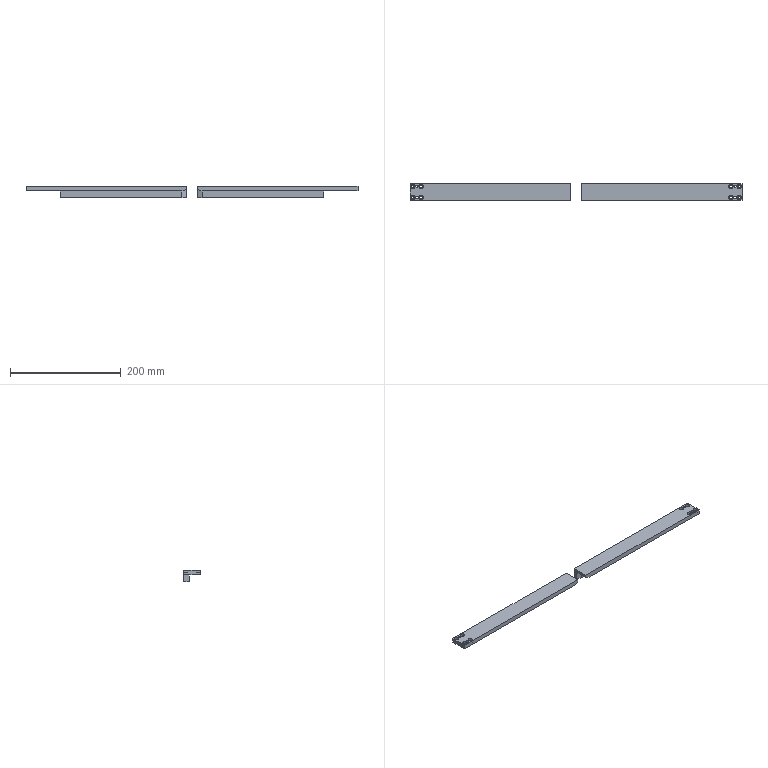NC program | NX | posted with a generic post | part box 600 x 30 x 20 mm
Lines 1 to 376 of 2978:
N10 G17 G21 G94 G90
(FLOOR_WALL , TOOL : D50)
N12 T01 M6
N14 G54
N16 G17 G0 G90 X-176. Y0. S6500 M3
N18 G43 Z30. H1
N20 Z3.
N22 G94 G1 Z0. F1250.
N24 X-173.
N26 X173.
N28 X176.
N30 Z3.
N32 G0 Z30.
N34 M5
(DRILLING_COPY_1 , TOOL : D6A45)
N36 T02 M6
N38 G54
N40 G17 G0 G90 X-140. Y-10. S3000 M3
N42 G43 Z30. H2
N44 G94 G81 G98 Z-1.6 F200. R3.
N46 X-132.5 Y-9.5
N48 X-125. Y-10.
N50 Y10.
N52 X-132.5
N54 X-140.
N56 G80
N58 G0 X-140. Y10. Z30.
N60 M5
(DRILLING_COPY_1_COPY_COPY_1_COPY_1_COPY , TOOL : 4.5ZT)
N62 T14 M6
N64 G54
N66 G17 G0 G90 X-140. Y10. S2000 M3
N68 G43 Z30. H14
N70 G94 G83 G98 Z-10.852 F120. Q2. R3.
N72 X-125.
N74 X-140. Y-10.
N76 X-125.
N78 G80
N80 G0 X-125. Y-10. Z30.
N82 M5
(DRILLING_COPY_1_COPY_COPY_1_COPY_1_COPY_COPY , TOOL : 2.5ZT)
N84 T12 M6
N86 G54
N88 G17 G0 G90 X-132.5 Y10. S2000 M3
N90 G43 Z30. H12
N92 G94 G83 G98 Z-10.251 F120. Q2. R3.
N94 Y-9.5
N96 G80
N98 G0 X-132.5 Y-9.5 Z30.
N100 M5
(ZLEVEL_PROFILE , TOOL : D10)
N102 T03 M6
N104 G54
N106 G17 G0 G90 X-47.703 Y20.1 S7000 M3
N108 G43 Z30. H3
N110 Z1.5
N112 G94 G1 X0. Z-1. F1000.
N114 X145. F3000.
N116 G2 X150.1 Y15. R5.1
N118 G1 Y-15.
N120 G2 X145. Y-20.1 R5.1
N122 G1 X-145.
N124 G2 X-150.1 Y-15. R5.1
N126 G1 Y15.
N128 G2 X-145. Y20.1 R5.1
N130 G1 X0.
N132 X57.29 Z-2.
N134 X145.
N136 G2 X150.1 Y15. R5.1
N138 G1 Y-15.
N140 G2 X145. Y-20.1 R5.1
N142 G1 X-145.
N144 G2 X-150.1 Y-15. R5.1
N146 G1 Y15.
N148 G2 X-145. Y20.1 R5.1
N150 G1 X0.
N152 X57.29 Z-3.
N154 X145.
N156 G2 X150.1 Y15. R5.1
N158 G1 Y-15.
N160 G2 X145. Y-20.1 R5.1
N162 G1 X-145.
N164 G2 X-150.1 Y-15. R5.1
N166 G1 Y15.
N168 G2 X-145. Y20.1 R5.1
N170 G1 X0.
N172 X57.29 Z-4.
N174 X145.
N176 G2 X150.1 Y15. R5.1
N178 G1 Y-15.
N180 G2 X145. Y-20.1 R5.1
N182 G1 X-145.
N184 G2 X-150.1 Y-15. R5.1
N186 G1 Y15.
N188 G2 X-145. Y20.1 R5.1
N190 G1 X0.
N192 X57.29 Z-5.
N194 X145.
N196 G2 X150.1 Y15. R5.1
N198 G1 Y-15.
N200 G2 X145. Y-20.1 R5.1
N202 G1 X-145.
N204 G2 X-150.1 Y-15. R5.1
N206 G1 Y15.
N208 G2 X-145. Y20.1 R5.1
N210 G1 X0.
N212 X57.29 Z-6.
N214 X145.
N216 G2 X150.1 Y15. R5.1
N218 G1 Y-15.
N220 G2 X145. Y-20.1 R5.1
N222 G1 X-145.
N224 G2 X-150.1 Y-15. R5.1
N226 G1 Y15.
N228 G2 X-145. Y20.1 R5.1
N230 G1 X0.
N232 X57.29 Z-7.
N234 X145.
N236 G2 X150.1 Y15. R5.1
N238 G1 Y-15.
N240 G2 X145. Y-20.1 R5.1
N242 G1 X-145.
N244 G2 X-150.1 Y-15. R5.1
N246 G1 Y15.
N248 G2 X-145. Y20.1 R5.1
N250 G1 X0.
N252 X57.29 Z-8.
N254 X145.
N256 G2 X150.1 Y15. R5.1
N258 G1 Y-15.
N260 G2 X145. Y-20.1 R5.1
N262 G1 X-145.
N264 G2 X-150.1 Y-15. R5.1
N266 G1 Y15.
N268 G2 X-145. Y20.1 R5.1
N270 G1 X0.
N272 X57.29 Z-9.
N274 X145.
N276 G2 X150.1 Y15. R5.1
N278 G1 Y-15.
N280 G2 X145. Y-20.1 R5.1
N282 G1 X-145.
N284 G2 X-150.1 Y-15. R5.1
N286 G1 Y15.
N288 G2 X-145. Y20.1 R5.1
N290 G1 X0.
N292 X57.29 Z-10.
N294 X145.
N296 G2 X150.1 Y15. R5.1
N298 G1 Y-15.
N300 G2 X145. Y-20.1 R5.1
N302 G1 X-145.
N304 G2 X-150.1 Y-15. R5.1
N306 G1 Y15.
N308 G2 X-145. Y20.1 R5.1
N310 G1 X0.
N312 X57.29 Z-11.
N314 X145.
N316 G2 X150.1 Y15. R5.1
N318 G1 Y-15.
N320 G2 X145. Y-20.1 R5.1
N322 G1 X-145.
N324 G2 X-150.1 Y-15. R5.1
N326 G1 Y15.
N328 G2 X-145. Y20.1 R5.1
N330 G1 X0.
N332 X57.29 Z-12.
N334 X145.
N336 G2 X150.1 Y15. R5.1
N338 G1 Y-15.
N340 G2 X145. Y-20.1 R5.1
N342 G1 X-145.
N344 G2 X-150.1 Y-15. R5.1
N346 G1 Y15.
N348 G2 X-145. Y20.1 R5.1
N350 G1 X0.
N352 X57.29 Z-13.
N354 X145.
N356 G2 X150.1 Y15. R5.1
N358 G1 Y-15.
N360 G2 X145. Y-20.1 R5.1
N362 G1 X-145.
N364 G2 X-150.1 Y-15. R5.1
N366 G1 Y15.
N368 G2 X-145. Y20.1 R5.1
N370 G1 X0.
N372 X57.29 Z-14.
N374 X145.
N376 G2 X150.1 Y15. R5.1
N378 G1 Y-15.
N380 G2 X145. Y-20.1 R5.1
N382 G1 X-145.
N384 G2 X-150.1 Y-15. R5.1
N386 G1 Y15.
N388 G2 X-145. Y20.1 R5.1
N390 G1 X0.
N392 X57.29 Z-15.
N394 X145.
N396 G2 X150.1 Y15. R5.1
N398 G1 Y-15.
N400 G2 X145. Y-20.1 R5.1
N402 G1 X-145.
N404 G2 X-150.1 Y-15. R5.1
N406 G1 Y15.
N408 G2 X-145. Y20.1 R5.1
N410 G1 X0.
N412 X57.29 Z-16.
N414 X145.
N416 G2 X150.1 Y15. R5.1
N418 G1 Y-15.
N420 G2 X145. Y-20.1 R5.1
N422 G1 X-145.
N424 G2 X-150.1 Y-15. R5.1
N426 G1 Y15.
N428 G2 X-145. Y20.1 R5.1
N430 G1 X0.
N432 X57.29 Z-17.
N434 X145.
N436 G2 X150.1 Y15. R5.1
N438 G1 Y-15.
N440 G2 X145. Y-20.1 R5.1
N442 G1 X-145.
N444 G2 X-150.1 Y-15. R5.1
N446 G1 Y15.
N448 G2 X-145. Y20.1 R5.1
N450 G1 X0.
N452 X57.29 Z-18.
N454 X145.
N456 G2 X150.1 Y15. R5.1
N458 G1 Y-15.
N460 G2 X145. Y-20.1 R5.1
N462 G1 X-145.
N464 G2 X-150.1 Y-15. R5.1
N466 G1 Y15.
N468 G2 X-145. Y20.1 R5.1
N470 G1 X0.
N472 X57.29 Z-19.
N474 X145.
N476 G2 X150.1 Y15. R5.1
N478 G1 Y-15.
N480 G2 X145. Y-20.1 R5.1
N482 G1 X-145.
N484 G2 X-150.1 Y-15. R5.1
N486 G1 Y15.
N488 G2 X-145. Y20.1 R5.1
N490 G1 X0.
N492 X57.29 Z-20.
N494 X145.
N496 G2 X150.1 Y15. R5.1
N498 G1 Y-15.
N500 G2 X145. Y-20.1 R5.1
N502 G1 X-145.
N504 G2 X-150.1 Y-15. R5.1
N506 G1 Y15.
N508 G2 X-145. Y20.1 R5.1
N510 G1 X57.29
N512 Z-18.5
N514 G0 Z30.
N516 M5
(ZLEVEL_PROFILE_COPY_COPY_1_COPY_COPY_COPY_1 , TOOL : D10JING)
N518 T04 M6
N520 G54
N522 G17 G0 G90 X146.096 Y-20.899 S7000 M3
N524 G43 Z30. H4
N526 Z-20.
N528 G94 G1 X145.866 Y-20.5 F1000.
N530 G3 X145. Y-20. R1.
N532 G1 X-145.
N534 G2 X-150. Y-15. R5.
N536 G1 Y15.
N538 G2 X-145. Y20. R5.
N540 G1 X145.
N542 G2 X150. Y15. R5.
N544 G1 Y-15.
N546 G2 X145. Y-20. R5.
N548 G3 X144.134 Y-20.5 R1.
N550 G1 X143.845 Y-21.
N552 G0 Z30.
N554 M5
(HOLE_MILLING_1 , TOOL : D6)
N556 T08 M6
N558 G54
N560 G17 G0 G90 X-140. Y10. S7000 M3
N562 G43 Z30. H8
N564 Z0.5
N566 G94 G3 X-139.5 Y9.5 R0.5 F1500.
N568 X-139. Y10. R0.5
N570 X-139. Y10. Z0. I-1. J0.
N572 X-139. Y10. Z-0.5 I-1. J0.
N574 X-139. Y10. Z-1. I-1. J0.
N576 X-139. Y10. Z-1.5 I-1. J0.
N578 X-139. Y10. Z-2. I-1. J0.
N580 X-139. Y10. Z-2.5 I-1. J0.
N582 X-139. Y10. Z-3. I-1. J0.
N584 X-139. Y10. Z-3.5 I-1. J0.
N586 X-139. Y10. Z-4. I-1. J0.
N588 X-139.691 Y9.049 Z-4.4 R-1.
N590 X-139.049 Y10.309 R1.
N592 X-139.691 Y9.049 R-1.
N594 X-139.37 Y9.679 R0.5
N596 X-140. Y10. R0.5
N598 G0 Z30.
N600 X-125.
N602 Z0.5
N604 G3 X-124.5 Y9.5 R0.5
N606 X-124. Y10. R0.5
N608 X-124. Y10. Z0. I-1. J0.
N610 X-124. Y10. Z-0.5 I-1. J0.
N612 X-124. Y10. Z-1. I-1. J0.
N614 X-124. Y10. Z-1.5 I-1. J0.
N616 X-124. Y10. Z-2. I-1. J0.
N618 X-124. Y10. Z-2.5 I-1. J0.
N620 X-124. Y10. Z-3. I-1. J0.
N622 X-124. Y10. Z-3.5 I-1. J0.
N624 X-124. Y10. Z-4. I-1. J0.
N626 X-124.691 Y9.049 Z-4.4 R-1.
N628 X-124.049 Y10.309 R1.
N630 X-124.691 Y9.049 R-1.
N632 X-124.37 Y9.679 R0.5
N634 X-125. Y10. R0.5
N636 G0 Z30.
N638 Y-10.
N640 Z0.5
N642 G3 X-124.5 Y-10.5 R0.5
N644 X-124. Y-10. R0.5
N646 X-124. Y-10. Z0. I-1. J0.
N648 X-124. Y-10. Z-0.5 I-1. J0.
N650 X-124. Y-10. Z-1. I-1. J0.
N652 X-124. Y-10. Z-1.5 I-1. J0.
N654 X-124. Y-10. Z-2. I-1. J0.
N656 X-124. Y-10. Z-2.5 I-1. J0.
N658 X-124. Y-10. Z-3. I-1. J0.
N660 X-124. Y-10. Z-3.5 I-1. J0.
N662 X-124. Y-10. Z-4. I-1. J0.
N664 X-124.691 Y-10.951 Z-4.4 R-1.
N666 X-124.049 Y-9.691 R1.
N668 X-124.691 Y-10.951 R-1.
N670 X-124.37 Y-10.321 R0.5
N672 X-125. Y-10. R0.5
N674 G0 Z30.
N676 X-140.
N678 Z0.5
N680 G3 X-139.5 Y-10.5 R0.5
N682 X-139. Y-10. R0.5
N684 X-139. Y-10. Z0. I-1. J0.
N686 X-139. Y-10. Z-0.5 I-1. J0.
N688 X-139. Y-10. Z-1. I-1. J0.
N690 X-139. Y-10. Z-1.5 I-1. J0.
N692 X-139. Y-10. Z-2. I-1. J0.
N694 X-139. Y-10. Z-2.5 I-1. J0.
N696 X-139. Y-10. Z-3. I-1. J0.
N698 X-139. Y-10. Z-3.5 I-1. J0.
N700 X-139. Y-10. Z-4. I-1. J0.
N702 X-139.691 Y-10.951 Z-4.4 R-1.
N704 X-139.049 Y-9.691 R1.
N706 X-139.691 Y-10.951 R-1.
N708 X-139.37 Y-10.321 R0.5
N710 X-140. Y-10. R0.5
N712 G0 Z30.
N714 M5